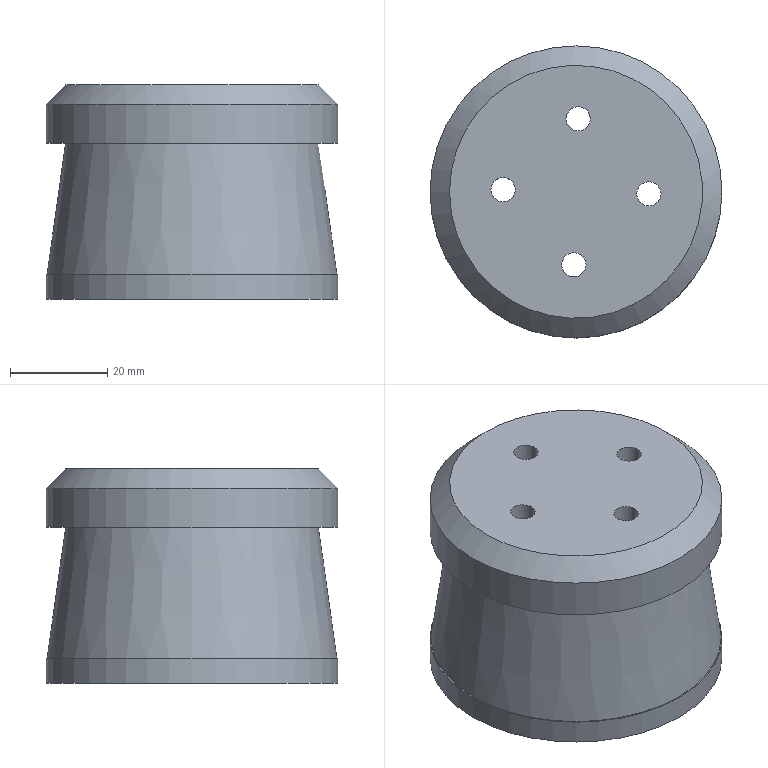Part | NX | features BREP 1 | 1 solid | 15 faces | box 60 x 60 x 44 mm | volume 55505 mm3 | cylinder 7 | plane 6 | cone 2 | commonest cylinder face diameters 5 x4 60 x2 45 x1
STEP:
#1=CARTESIAN_POINT('',(-14.142,-17.5,-44.));
#2=VERTEX_POINT('',#1);
#3=CARTESIAN_POINT('',(14.142,-17.5,-44.));
#4=VERTEX_POINT('',#3);
#5=CARTESIAN_POINT('',(0.,0.,-44.));
#6=DIRECTION('',(0.,0.,-1.));
#7=DIRECTION('',(-1.,0.,0.));
#8=AXIS2_PLACEMENT_3D('',#5,#6,#7);
#9=CIRCLE('',#8,22.5);
#10=EDGE_CURVE('',#2,#4,#9,.T.);
#11=ORIENTED_EDGE('',*,*,#10,.F.);
#12=CARTESIAN_POINT('',(-14.142,-17.5,-82.));
#13=VERTEX_POINT('',#12);
#14=CARTESIAN_POINT('',(-14.142,-17.5,-82.));
#15=DIRECTION('',(0.,0.,1.));
#16=VECTOR('',#15,1000.);
#17=LINE('',#14,#16);
#18=EDGE_CURVE('',#13,#2,#17,.T.);
#19=ORIENTED_EDGE('',*,*,#18,.F.);
#20=CARTESIAN_POINT('',(14.142,-17.5,-82.));
#21=VERTEX_POINT('',#20);
#22=CARTESIAN_POINT('',(0.,0.,-82.));
#23=DIRECTION('',(0.,0.,-1.));
#24=DIRECTION('',(-1.,0.,0.));
#25=AXIS2_PLACEMENT_3D('',#22,#23,#24);
#26=CIRCLE('',#25,22.5);
#27=EDGE_CURVE('',#13,#21,#26,.T.);
#28=ORIENTED_EDGE('',*,*,#27,.T.);
#29=CARTESIAN_POINT('',(14.142,-17.5,-82.));
#30=DIRECTION('',(0.,0.,-1.));
#31=VECTOR('',#30,1000.);
#32=LINE('',#29,#31);
#33=EDGE_CURVE('',#4,#21,#32,.T.);
#34=ORIENTED_EDGE('',*,*,#33,.F.);
#35=EDGE_LOOP('',(#11,#19,#28,#34));
#36=FACE_BOUND('',#35,.T.);
#37=CARTESIAN_POINT('',(0.,0.,-82.));
#38=DIRECTION('',(0.,0.,1.));
#39=DIRECTION('',(-1.,0.,0.));
#40=AXIS2_PLACEMENT_3D('',#37,#38,#39);
#41=CYLINDRICAL_SURFACE('',#40,22.5);
#42=ADVANCED_FACE('',(#36),#41,.F.);
#43=CARTESIAN_POINT('',(-30.,0.,-77.));
#44=VERTEX_POINT('',#43);
#45=CARTESIAN_POINT('',(0.,0.,-77.));
#46=DIRECTION('',(0.,0.,-1.));
#47=DIRECTION('',(-1.,0.,0.));
#48=AXIS2_PLACEMENT_3D('',#45,#46,#47);
#49=CIRCLE('',#48,30.);
#50=EDGE_CURVE('',#44,#44,#49,.T.);
#51=ORIENTED_EDGE('',*,*,#50,.T.);
#52=EDGE_LOOP('',(#51));
#53=FACE_BOUND('',#52,.T.);
#54=CARTESIAN_POINT('',(30.,0.,-82.));
#55=VERTEX_POINT('',#54);
#56=CARTESIAN_POINT('',(0.,0.,-82.));
#57=DIRECTION('',(0.,0.,-1.));
#58=DIRECTION('',(1.,0.,0.));
#59=AXIS2_PLACEMENT_3D('',#56,#57,#58);
#60=CIRCLE('',#59,30.);
#61=EDGE_CURVE('',#55,#55,#60,.T.);
#62=ORIENTED_EDGE('',*,*,#61,.F.);
#63=EDGE_LOOP('',(#62));
#64=FACE_BOUND('',#63,.T.);
#65=CARTESIAN_POINT('',(0.,0.,-82.));
#66=DIRECTION('',(0.,0.,1.));
#67=DIRECTION('',(-1.,0.,0.));
#68=AXIS2_PLACEMENT_3D('',#65,#66,#67);
#69=CYLINDRICAL_SURFACE('',#68,30.);
#70=ADVANCED_FACE('',(#53,#64),#69,.T.);
#71=CARTESIAN_POINT('',(14.142,-17.5,-44.));
#72=DIRECTION('',(-1.,0.,0.));
#73=VECTOR('',#72,1000.);
#74=LINE('',#71,#73);
#75=EDGE_CURVE('',#4,#2,#74,.T.);
#76=ORIENTED_EDGE('',*,*,#75,.F.);
#77=ORIENTED_EDGE('',*,*,#33,.T.);
#78=CARTESIAN_POINT('',(14.142,-17.5,-82.));
#79=DIRECTION('',(-1.,0.,0.));
#80=VECTOR('',#79,1000.);
#81=LINE('',#78,#80);
#82=EDGE_CURVE('',#21,#13,#81,.T.);
#83=ORIENTED_EDGE('',*,*,#82,.T.);
#84=ORIENTED_EDGE('',*,*,#18,.T.);
#85=EDGE_LOOP('',(#76,#77,#83,#84));
#86=FACE_BOUND('',#85,.T.);
#87=CARTESIAN_POINT('',(14.142,-17.5,-82.));
#88=DIRECTION('',(0.,1.,0.));
#89=DIRECTION('',(0.,0.,-1.));
#90=AXIS2_PLACEMENT_3D('',#87,#88,#89);
#91=PLANE('',#90);
#92=ADVANCED_FACE('',(#86),#91,.T.);
#93=ORIENTED_EDGE('',*,*,#61,.T.);
#94=EDGE_LOOP('',(#93));
#95=FACE_BOUND('',#94,.T.);
#96=ORIENTED_EDGE('',*,*,#27,.F.);
#97=ORIENTED_EDGE('',*,*,#82,.F.);
#98=EDGE_LOOP('',(#96,#97));
#99=FACE_BOUND('',#98,.T.);
#100=CARTESIAN_POINT('',(0.,0.,-82.));
#101=DIRECTION('',(0.,0.,-1.));
#102=DIRECTION('',(1.,0.,0.));
#103=AXIS2_PLACEMENT_3D('',#100,#101,#102);
#104=PLANE('',#103);
#105=ADVANCED_FACE('',(#95,#99),#104,.T.);
#106=CARTESIAN_POINT('',(12.494,-0.4372,-44.));
#107=VERTEX_POINT('',#106);
#108=CARTESIAN_POINT('',(14.994,-0.4372,-44.));
#109=DIRECTION('',(0.,0.,1.));
#110=DIRECTION('',(-1.,0.,0.));
#111=AXIS2_PLACEMENT_3D('',#108,#109,#110);
#112=CIRCLE('',#111,2.5);
#113=EDGE_CURVE('',#107,#107,#112,.T.);
#114=ORIENTED_EDGE('',*,*,#113,.T.);
#115=EDGE_LOOP('',(#114));
#116=FACE_BOUND('',#115,.T.);
#117=CARTESIAN_POINT('',(-2.063,14.994,-44.));
#118=VERTEX_POINT('',#117);
#119=CARTESIAN_POINT('',(0.4372,14.994,-44.));
#120=DIRECTION('',(0.,0.,1.));
#121=DIRECTION('',(-1.,0.,0.));
#122=AXIS2_PLACEMENT_3D('',#119,#120,#121);
#123=CIRCLE('',#122,2.5);
#124=EDGE_CURVE('',#118,#118,#123,.T.);
#125=ORIENTED_EDGE('',*,*,#124,.T.);
#126=EDGE_LOOP('',(#125));
#127=FACE_BOUND('',#126,.T.);
#128=CARTESIAN_POINT('',(-2.937,-14.994,-44.));
#129=VERTEX_POINT('',#128);
#130=CARTESIAN_POINT('',(-0.4372,-14.994,-44.));
#131=DIRECTION('',(0.,0.,1.));
#132=DIRECTION('',(-1.,0.,0.));
#133=AXIS2_PLACEMENT_3D('',#130,#131,#132);
#134=CIRCLE('',#133,2.5);
#135=EDGE_CURVE('',#129,#129,#134,.T.);
#136=ORIENTED_EDGE('',*,*,#135,.T.);
#137=EDGE_LOOP('',(#136));
#138=FACE_BOUND('',#137,.T.);
#139=CARTESIAN_POINT('',(-17.494,0.4372,-44.));
#140=VERTEX_POINT('',#139);
#141=CARTESIAN_POINT('',(-14.994,0.4372,-44.));
#142=DIRECTION('',(0.,0.,1.));
#143=DIRECTION('',(-1.,0.,0.));
#144=AXIS2_PLACEMENT_3D('',#141,#142,#143);
#145=CIRCLE('',#144,2.5);
#146=EDGE_CURVE('',#140,#140,#145,.T.);
#147=ORIENTED_EDGE('',*,*,#146,.T.);
#148=EDGE_LOOP('',(#147));
#149=FACE_BOUND('',#148,.T.);
#150=ORIENTED_EDGE('',*,*,#75,.T.);
#151=ORIENTED_EDGE('',*,*,#10,.T.);
#152=EDGE_LOOP('',(#150,#151));
#153=FACE_BOUND('',#152,.T.);
#154=CARTESIAN_POINT('',(0.,0.,-44.));
#155=DIRECTION('',(0.,0.,-1.));
#156=DIRECTION('',(1.,0.,0.));
#157=AXIS2_PLACEMENT_3D('',#154,#155,#156);
#158=PLANE('',#157);
#159=ADVANCED_FACE('',(#116,#127,#138,#149,#153),#158,.T.);
#160=CARTESIAN_POINT('',(-29.795,0.,-77.));
#161=VERTEX_POINT('',#160);
#162=CARTESIAN_POINT('',(0.,0.,-77.));
#163=DIRECTION('',(0.,0.,1.));
#164=DIRECTION('',(-1.,0.,0.));
#165=AXIS2_PLACEMENT_3D('',#162,#163,#164);
#166=CIRCLE('',#165,29.795);
#167=EDGE_CURVE('',#161,#161,#166,.T.);
#168=ORIENTED_EDGE('',*,*,#167,.F.);
#169=EDGE_LOOP('',(#168));
#170=FACE_BOUND('',#169,.T.);
#171=ORIENTED_EDGE('',*,*,#50,.F.);
#172=EDGE_LOOP('',(#171));
#173=FACE_BOUND('',#172,.T.);
#174=CARTESIAN_POINT('',(0.,0.,-77.));
#175=DIRECTION('',(0.,0.,-1.));
#176=DIRECTION('',(1.,0.,0.));
#177=AXIS2_PLACEMENT_3D('',#174,#175,#176);
#178=PLANE('',#177);
#179=ADVANCED_FACE('',(#170,#173),#178,.F.);
#180=CARTESIAN_POINT('',(-26.,0.,-50.));
#181=VERTEX_POINT('',#180);
#182=CARTESIAN_POINT('',(0.,0.,-50.));
#183=DIRECTION('',(0.,0.,1.));
#184=DIRECTION('',(-1.,0.,0.));
#185=AXIS2_PLACEMENT_3D('',#182,#183,#184);
#186=CIRCLE('',#185,26.);
#187=EDGE_CURVE('',#181,#181,#186,.T.);
#188=ORIENTED_EDGE('',*,*,#187,.T.);
#189=EDGE_LOOP('',(#188));
#190=FACE_BOUND('',#189,.T.);
#191=CARTESIAN_POINT('',(-30.,0.,-50.));
#192=VERTEX_POINT('',#191);
#193=CARTESIAN_POINT('',(0.,0.,-50.));
#194=DIRECTION('',(0.,0.,-1.));
#195=DIRECTION('',(-1.,0.,0.));
#196=AXIS2_PLACEMENT_3D('',#193,#194,#195);
#197=CIRCLE('',#196,30.);
#198=EDGE_CURVE('',#192,#192,#197,.T.);
#199=ORIENTED_EDGE('',*,*,#198,.T.);
#200=EDGE_LOOP('',(#199));
#201=FACE_BOUND('',#200,.T.);
#202=CARTESIAN_POINT('',(0.,0.,-50.));
#203=DIRECTION('',(0.,0.,-1.));
#204=DIRECTION('',(1.,0.,0.));
#205=AXIS2_PLACEMENT_3D('',#202,#203,#204);
#206=PLANE('',#205);
#207=ADVANCED_FACE('',(#190,#201),#206,.T.);
#208=ORIENTED_EDGE('',*,*,#167,.T.);
#209=EDGE_LOOP('',(#208));
#210=FACE_BOUND('',#209,.T.);
#211=ORIENTED_EDGE('',*,*,#187,.F.);
#212=EDGE_LOOP('',(#211));
#213=FACE_BOUND('',#212,.T.);
#214=CARTESIAN_POINT('',(0.,0.,-50.));
#215=DIRECTION('',(0.,0.,-1.));
#216=DIRECTION('',(1.,0.,0.));
#217=AXIS2_PLACEMENT_3D('',#214,#215,#216);
#218=CONICAL_SURFACE('',#217,26.,0.1396);
#219=ADVANCED_FACE('',(#210,#213),#218,.T.);
#220=CARTESIAN_POINT('',(12.494,-0.4372,-38.));
#221=VERTEX_POINT('',#220);
#222=CARTESIAN_POINT('',(14.994,-0.4372,-38.));
#223=DIRECTION('',(0.,0.,1.));
#224=DIRECTION('',(-1.,0.,0.));
#225=AXIS2_PLACEMENT_3D('',#222,#223,#224);
#226=CIRCLE('',#225,2.5);
#227=EDGE_CURVE('',#221,#221,#226,.T.);
#228=ORIENTED_EDGE('',*,*,#227,.F.);
#229=EDGE_LOOP('',(#228));
#230=FACE_BOUND('',#229,.T.);
#231=CARTESIAN_POINT('',(-2.063,14.994,-38.));
#232=VERTEX_POINT('',#231);
#233=CARTESIAN_POINT('',(0.4372,14.994,-38.));
#234=DIRECTION('',(0.,0.,1.));
#235=DIRECTION('',(-1.,0.,0.));
#236=AXIS2_PLACEMENT_3D('',#233,#234,#235);
#237=CIRCLE('',#236,2.5);
#238=EDGE_CURVE('',#232,#232,#237,.T.);
#239=ORIENTED_EDGE('',*,*,#238,.F.);
#240=EDGE_LOOP('',(#239));
#241=FACE_BOUND('',#240,.T.);
#242=CARTESIAN_POINT('',(-2.937,-14.994,-38.));
#243=VERTEX_POINT('',#242);
#244=CARTESIAN_POINT('',(-0.4372,-14.994,-38.));
#245=DIRECTION('',(0.,0.,1.));
#246=DIRECTION('',(-1.,0.,0.));
#247=AXIS2_PLACEMENT_3D('',#244,#245,#246);
#248=CIRCLE('',#247,2.5);
#249=EDGE_CURVE('',#243,#243,#248,.T.);
#250=ORIENTED_EDGE('',*,*,#249,.F.);
#251=EDGE_LOOP('',(#250));
#252=FACE_BOUND('',#251,.T.);
#253=CARTESIAN_POINT('',(-17.494,0.4372,-38.));
#254=VERTEX_POINT('',#253);
#255=CARTESIAN_POINT('',(-14.994,0.4372,-38.));
#256=DIRECTION('',(0.,0.,1.));
#257=DIRECTION('',(-1.,0.,0.));
#258=AXIS2_PLACEMENT_3D('',#255,#256,#257);
#259=CIRCLE('',#258,2.5);
#260=EDGE_CURVE('',#254,#254,#259,.T.);
#261=ORIENTED_EDGE('',*,*,#260,.F.);
#262=EDGE_LOOP('',(#261));
#263=FACE_BOUND('',#262,.T.);
#264=CARTESIAN_POINT('',(-26.,0.,-38.));
#265=VERTEX_POINT('',#264);
#266=CARTESIAN_POINT('',(0.,0.,-38.));
#267=DIRECTION('',(0.,0.,1.));
#268=DIRECTION('',(-1.,0.,0.));
#269=AXIS2_PLACEMENT_3D('',#266,#267,#268);
#270=CIRCLE('',#269,26.);
#271=EDGE_CURVE('',#265,#265,#270,.T.);
#272=ORIENTED_EDGE('',*,*,#271,.T.);
#273=EDGE_LOOP('',(#272));
#274=FACE_BOUND('',#273,.T.);
#275=CARTESIAN_POINT('',(0.,0.,-38.));
#276=DIRECTION('',(0.,0.,-1.));
#277=DIRECTION('',(1.,0.,0.));
#278=AXIS2_PLACEMENT_3D('',#275,#276,#277);
#279=PLANE('',#278);
#280=ADVANCED_FACE('',(#230,#241,#252,#263,#274),#279,.F.);
#281=ORIENTED_EDGE('',*,*,#271,.F.);
#282=EDGE_LOOP('',(#281));
#283=FACE_BOUND('',#282,.T.);
#284=CARTESIAN_POINT('',(-30.,0.,-42.));
#285=VERTEX_POINT('',#284);
#286=CARTESIAN_POINT('',(0.,0.,-42.));
#287=DIRECTION('',(0.,0.,-1.));
#288=DIRECTION('',(-1.,0.,0.));
#289=AXIS2_PLACEMENT_3D('',#286,#287,#288);
#290=CIRCLE('',#289,30.);
#291=EDGE_CURVE('',#285,#285,#290,.T.);
#292=ORIENTED_EDGE('',*,*,#291,.F.);
#293=EDGE_LOOP('',(#292));
#294=FACE_BOUND('',#293,.T.);
#295=CARTESIAN_POINT('',(0.,0.,-42.));
#296=DIRECTION('',(0.,0.,-1.));
#297=DIRECTION('',(1.,0.,0.));
#298=AXIS2_PLACEMENT_3D('',#295,#296,#297);
#299=CONICAL_SURFACE('',#298,30.,0.7854);
#300=ADVANCED_FACE('',(#283,#294),#299,.T.);
#301=ORIENTED_EDGE('',*,*,#291,.T.);
#302=EDGE_LOOP('',(#301));
#303=FACE_BOUND('',#302,.T.);
#304=ORIENTED_EDGE('',*,*,#198,.F.);
#305=EDGE_LOOP('',(#304));
#306=FACE_BOUND('',#305,.T.);
#307=CARTESIAN_POINT('',(0.,0.,-82.));
#308=DIRECTION('',(0.,0.,1.));
#309=DIRECTION('',(-1.,0.,0.));
#310=AXIS2_PLACEMENT_3D('',#307,#308,#309);
#311=CYLINDRICAL_SURFACE('',#310,30.);
#312=ADVANCED_FACE('',(#303,#306),#311,.T.);
#313=ORIENTED_EDGE('',*,*,#146,.F.);
#314=EDGE_LOOP('',(#313));
#315=FACE_BOUND('',#314,.T.);
#316=ORIENTED_EDGE('',*,*,#260,.T.);
#317=EDGE_LOOP('',(#316));
#318=FACE_BOUND('',#317,.T.);
#319=CARTESIAN_POINT('',(-14.994,0.4372,1.));
#320=DIRECTION('',(0.,0.,-1.));
#321=DIRECTION('',(1.,0.,0.));
#322=AXIS2_PLACEMENT_3D('',#319,#320,#321);
#323=CYLINDRICAL_SURFACE('',#322,2.5);
#324=ADVANCED_FACE('',(#315,#318),#323,.F.);
#325=ORIENTED_EDGE('',*,*,#135,.F.);
#326=EDGE_LOOP('',(#325));
#327=FACE_BOUND('',#326,.T.);
#328=ORIENTED_EDGE('',*,*,#249,.T.);
#329=EDGE_LOOP('',(#328));
#330=FACE_BOUND('',#329,.T.);
#331=CARTESIAN_POINT('',(-0.4372,-14.994,1.));
#332=DIRECTION('',(0.,0.,-1.));
#333=DIRECTION('',(1.,0.,0.));
#334=AXIS2_PLACEMENT_3D('',#331,#332,#333);
#335=CYLINDRICAL_SURFACE('',#334,2.5);
#336=ADVANCED_FACE('',(#327,#330),#335,.F.);
#337=ORIENTED_EDGE('',*,*,#124,.F.);
#338=EDGE_LOOP('',(#337));
#339=FACE_BOUND('',#338,.T.);
#340=ORIENTED_EDGE('',*,*,#238,.T.);
#341=EDGE_LOOP('',(#340));
#342=FACE_BOUND('',#341,.T.);
#343=CARTESIAN_POINT('',(0.4372,14.994,1.));
#344=DIRECTION('',(0.,0.,-1.));
#345=DIRECTION('',(1.,0.,0.));
#346=AXIS2_PLACEMENT_3D('',#343,#344,#345);
#347=CYLINDRICAL_SURFACE('',#346,2.5);
#348=ADVANCED_FACE('',(#339,#342),#347,.F.);
#349=ORIENTED_EDGE('',*,*,#113,.F.);
#350=EDGE_LOOP('',(#349));
#351=FACE_BOUND('',#350,.T.);
#352=ORIENTED_EDGE('',*,*,#227,.T.);
#353=EDGE_LOOP('',(#352));
#354=FACE_BOUND('',#353,.T.);
#355=CARTESIAN_POINT('',(14.994,-0.4372,1.));
#356=DIRECTION('',(0.,0.,-1.));
#357=DIRECTION('',(1.,0.,0.));
#358=AXIS2_PLACEMENT_3D('',#355,#356,#357);
#359=CYLINDRICAL_SURFACE('',#358,2.5);
#360=ADVANCED_FACE('',(#351,#354),#359,.F.);
#361=CLOSED_SHELL('',(#42,#70,#92,#105,#159,#179,#207,#219,#280,#300,#312,#324,#336,#348,#360));
#362=MANIFOLD_SOLID_BREP('',#361);
#363=(LENGTH_UNIT()NAMED_UNIT(*)SI_UNIT(.MILLI.,.METRE.));
#364=UNCERTAINTY_MEASURE_WITH_UNIT(LENGTH_MEASURE(0.00001),#363,'','');
#365=(NAMED_UNIT(*)PLANE_ANGLE_UNIT()SI_UNIT($,.RADIAN.));
#366=(NAMED_UNIT(*)SI_UNIT($,.STERADIAN.)SOLID_ANGLE_UNIT());
#367=(GEOMETRIC_REPRESENTATION_CONTEXT(3)GLOBAL_UNCERTAINTY_ASSIGNED_CONTEXT((#364))GLOBAL_UNIT_ASSIGNED_CONTEXT((#363,#365,#366))REPRESENTATION_CONTEXT('',''));
#368=ADVANCED_BREP_SHAPE_REPRESENTATION('',(#362),#367);